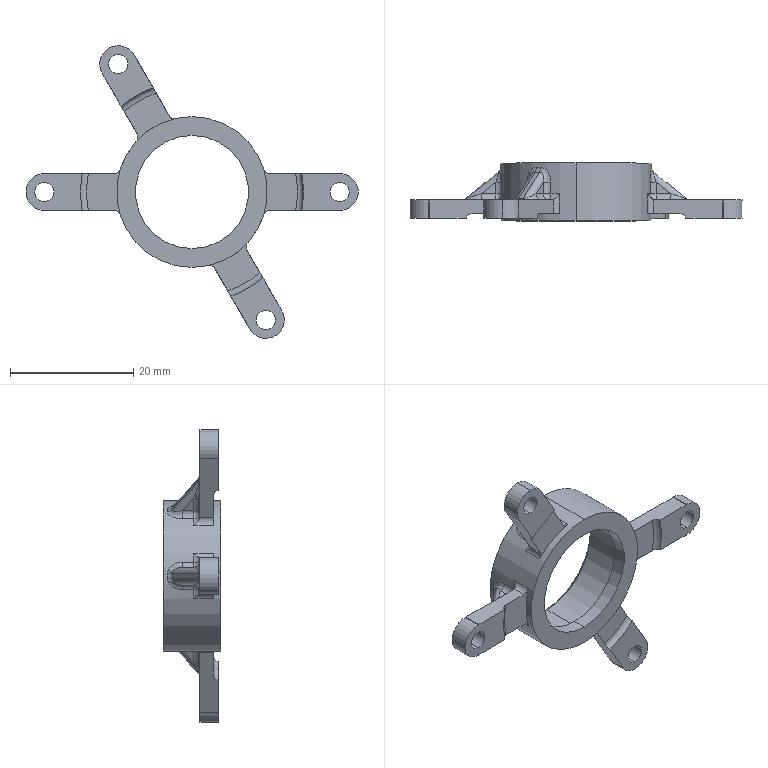Part | SolidWorks | features ICE 6, Fillet 2, BossThin 1, Chamfer 1, CirPattern 1, Extrusion 1, MirrorPattern 1, Rib 1 | 1 solid | 139 faces | box 54 x 9.4 x 47.569 mm | volume 2533 mm3 | cylinder 62 | plane 35 | spline 20 | torus 12 | sphere 8 | cone 2 | commonest cylinder face diameters 2 x39 6 x9 3.1 x8 18.4 x2 20.1 x2 24.5 x2